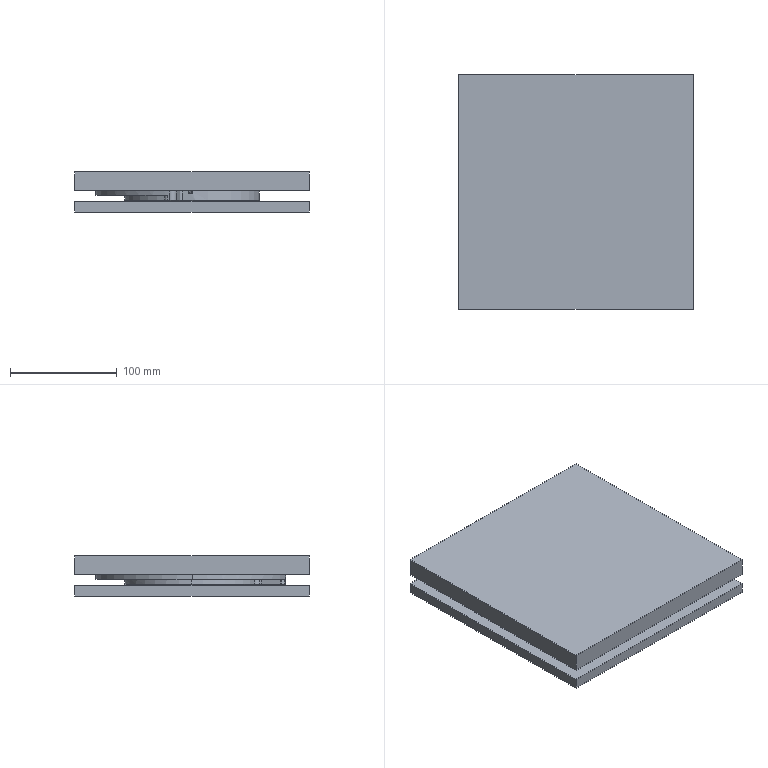Part | 3 solids | 216 faces | box 220 x 220 x 37.5 mm | volume 1348098 mm3 | cylinder 109 | cone 48 | plane 40 | spline 11 | sphere 4 | torus 4 | commonest cylinder face diameters 10 x14 3.5 x12 5 x12 2.5 x10 4 x10 6 x8